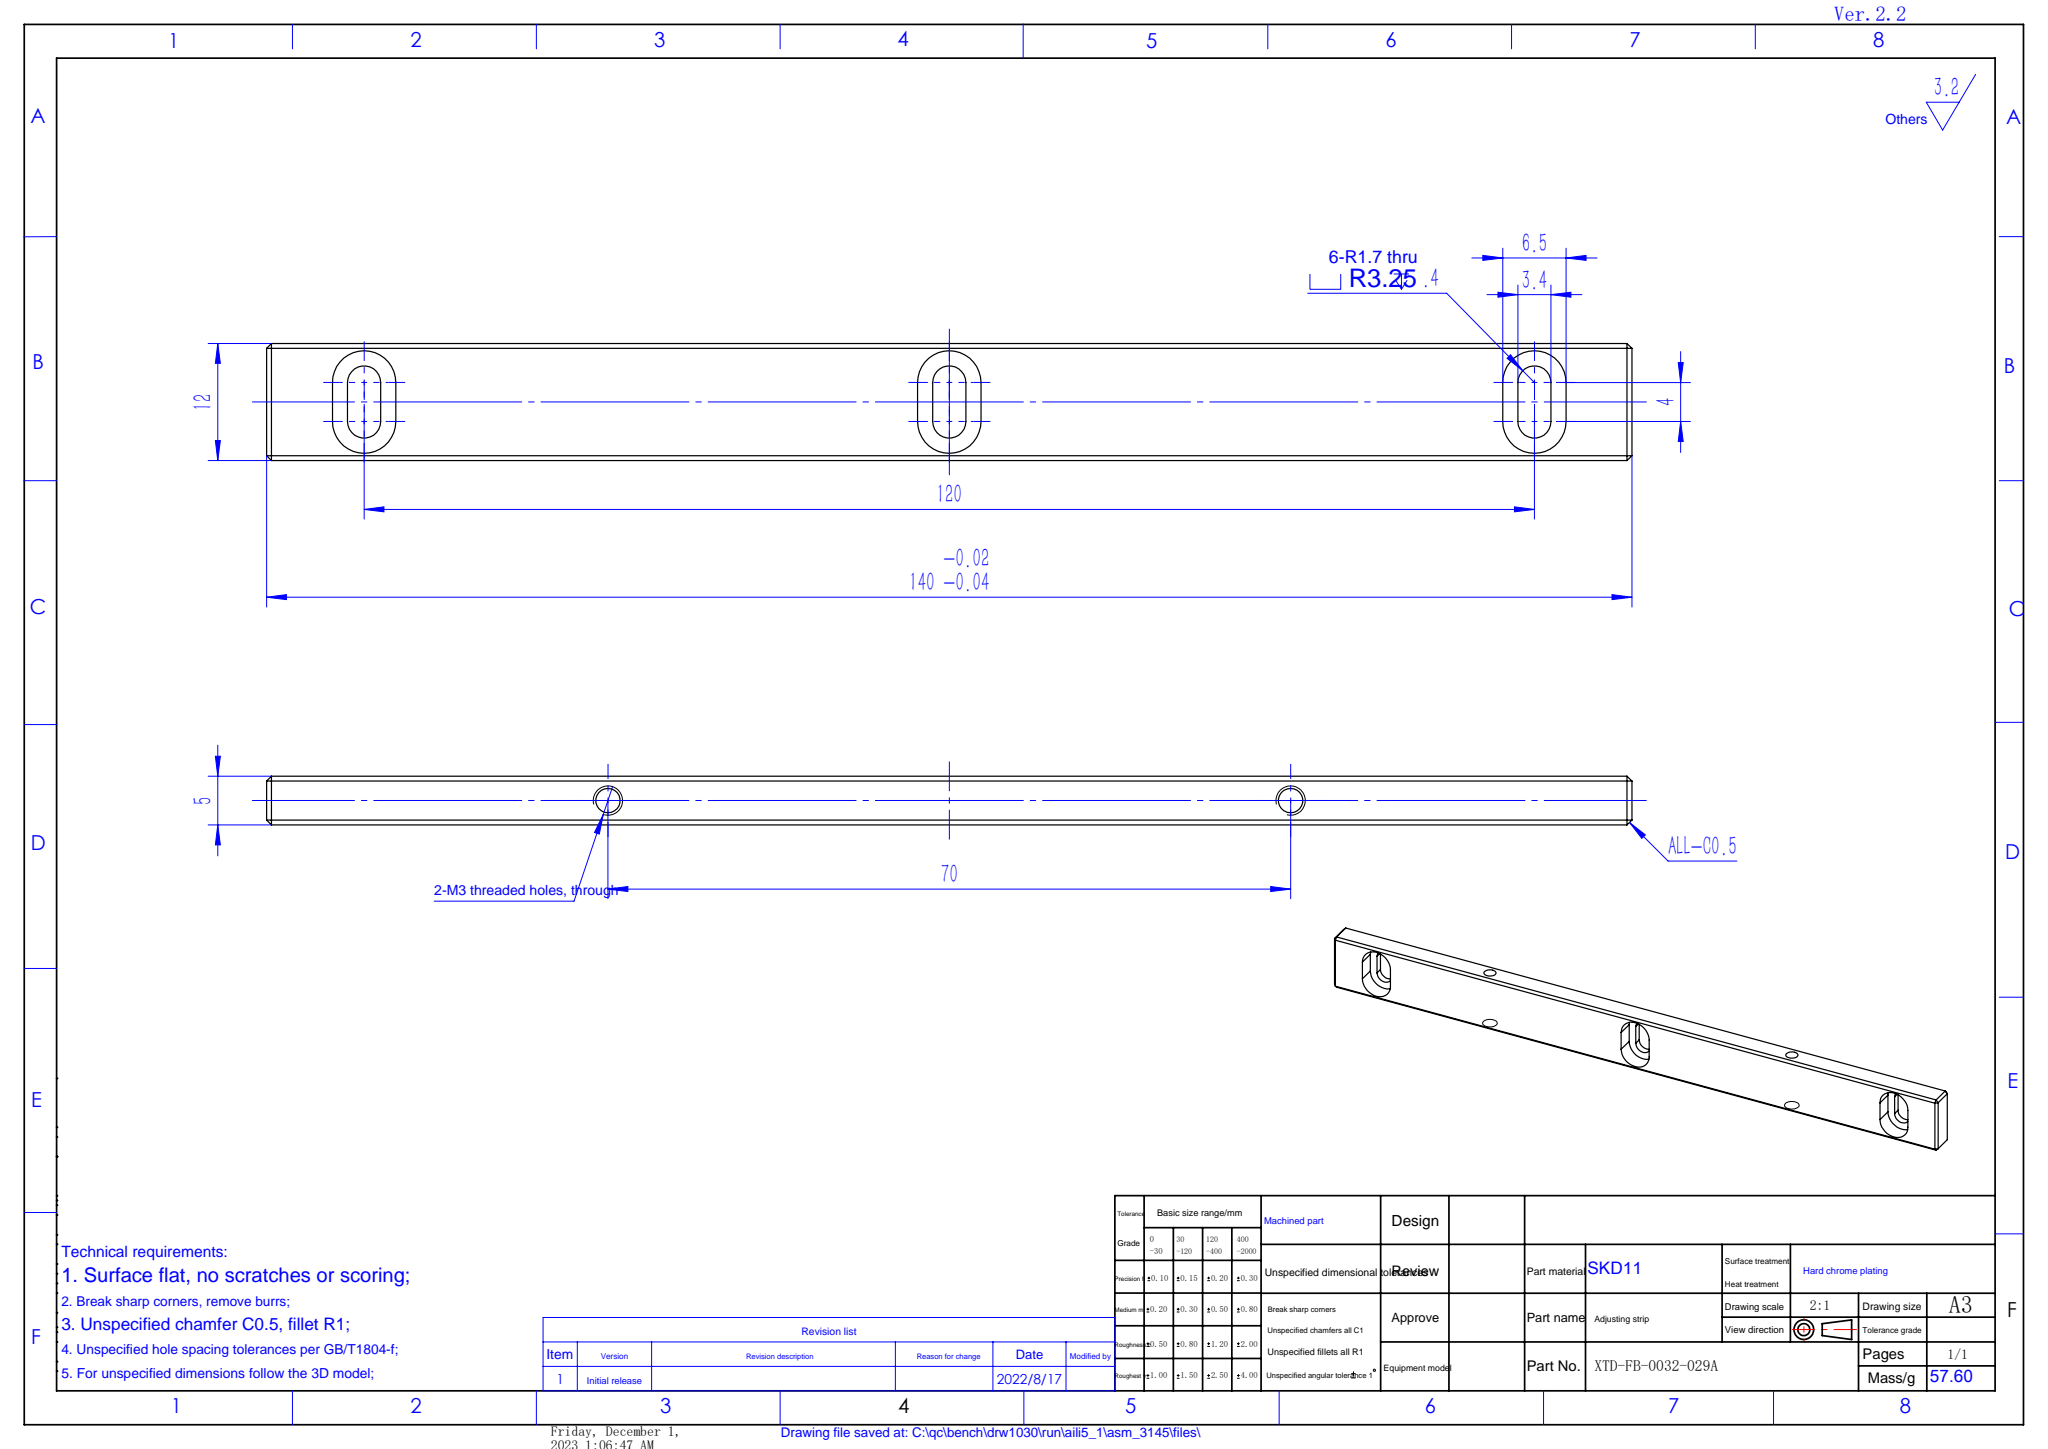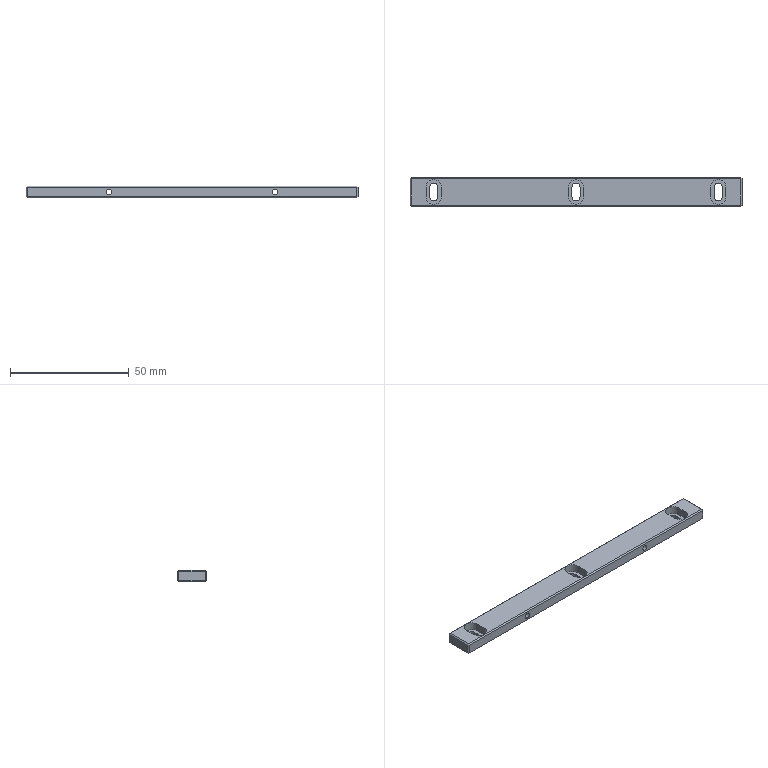Part | SolidWorks | features HoleWzd 2, Chamfer 1, Extrusion 1 | 1 solid | 57 faces | box 140 x 12 x 5 mm | volume 7481 mm3 | plane 41 | cylinder 16 | commonest cylinder face diameters 3.4 x6 6.5 x6 2.5 x4